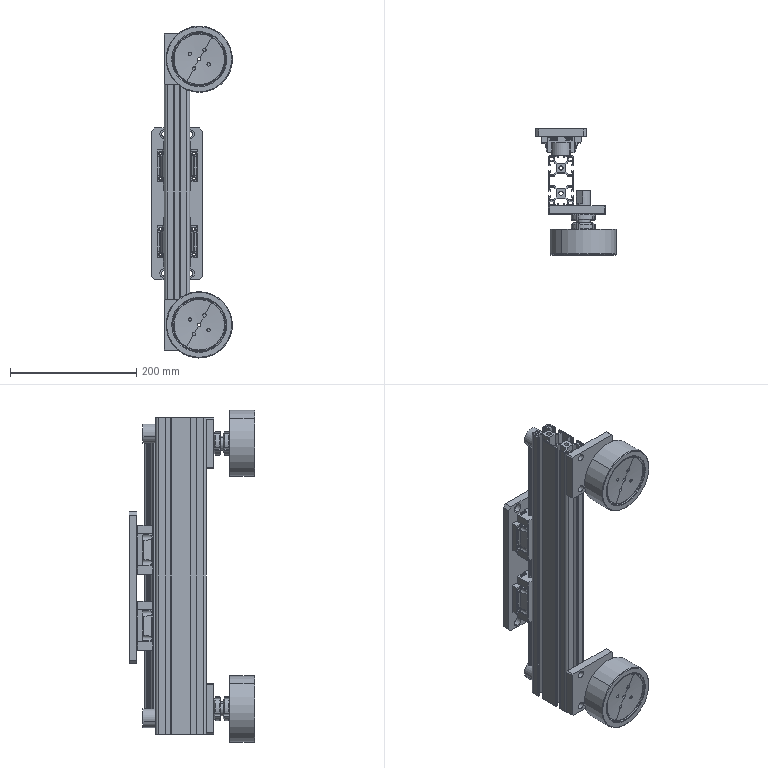Part | SolidWorks | 17 solids | 1454 faces | box 127.5 x 199 x 525 mm | volume 1466549 mm3 | plane 895 | cylinder 291 | spline 170 | cone 94 | torus 4 | commonest cylinder face diameters 1 x36 6 x30 2 x22 4.2 x16 5.2 x16 38 x16